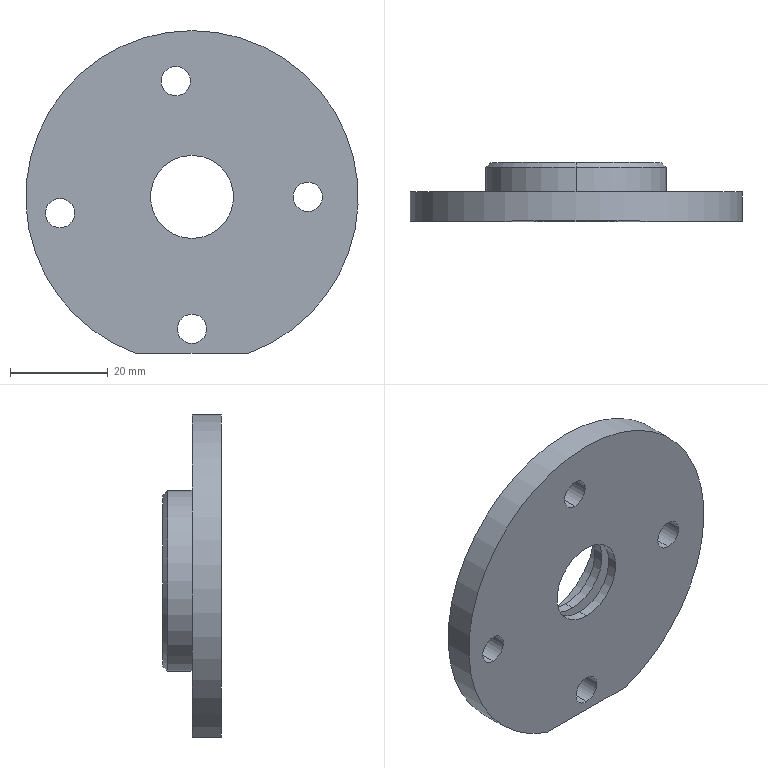Part | SolidWorks | features ICE 7, Chamfer 1, Extrusion 1, Fillet 1 | 1 solid | 30 faces | box 68 x 12 x 66 mm | volume 21544 mm3 | cylinder 19 | plane 7 | torus 2 | cone 2 | commonest cylinder face diameters 6 x8 17 x4 25 x2 29 x2 37 x2 68 x1
STEP:
#1=CARTESIAN_POINT('',(0.,0.,-30.));
#2=VERTEX_POINT('',#1);
#3=CARTESIAN_POINT('',(0.,0.,-24.));
#4=VERTEX_POINT('',#3);
#5=CARTESIAN_POINT('',(0.,0.,-27.));
#6=DIRECTION('',(0.,1.,0.));
#7=DIRECTION('',(0.,0.,1.));
#8=AXIS2_PLACEMENT_3D('',#5,#6,#7);
#9=CIRCLE('',#8,3.);
#10=EDGE_CURVE('',#2,#4,#9,.T.);
#11=ORIENTED_EDGE('',*,*,#10,.F.);
#12=CARTESIAN_POINT('',(0.,6.,-30.));
#13=VERTEX_POINT('',#12);
#14=CARTESIAN_POINT('',(0.,-74.,-30.));
#15=DIRECTION('',(0.,1.,0.));
#16=VECTOR('',#15,1000.);
#17=LINE('',#14,#16);
#18=EDGE_CURVE('',#2,#13,#17,.T.);
#19=ORIENTED_EDGE('',*,*,#18,.T.);
#20=CARTESIAN_POINT('',(0.,6.,-24.));
#21=VERTEX_POINT('',#20);
#22=CARTESIAN_POINT('',(0.,6.,-27.));
#23=DIRECTION('',(0.,1.,0.));
#24=DIRECTION('',(0.,0.,1.));
#25=AXIS2_PLACEMENT_3D('',#22,#23,#24);
#26=CIRCLE('',#25,3.);
#27=EDGE_CURVE('',#13,#21,#26,.T.);
#28=ORIENTED_EDGE('',*,*,#27,.T.);
#29=CARTESIAN_POINT('',(0.,-74.,-24.));
#30=DIRECTION('',(0.,1.,0.));
#31=VECTOR('',#30,1000.);
#32=LINE('',#29,#31);
#33=EDGE_CURVE('',#4,#21,#32,.T.);
#34=ORIENTED_EDGE('',*,*,#33,.F.);
#35=EDGE_LOOP('',(#11,#19,#28,#34));
#36=FACE_OUTER_BOUND('',#35,.T.);
#37=CARTESIAN_POINT('',(0.,-74.,-27.));
#38=DIRECTION('',(0.,1.,0.));
#39=DIRECTION('',(0.,0.,1.));
#40=AXIS2_PLACEMENT_3D('',#37,#38,#39);
#41=CYLINDRICAL_SURFACE('',#40,3.);
#42=ADVANCED_FACE('',(#36),#41,.F.);
#43=CARTESIAN_POINT('',(23.68,0.,-3.));
#44=VERTEX_POINT('',#43);
#45=CARTESIAN_POINT('',(23.68,0.,3.));
#46=VERTEX_POINT('',#45);
#47=CARTESIAN_POINT('',(23.68,0.,0.));
#48=DIRECTION('',(0.,1.,0.));
#49=DIRECTION('',(0.,0.,1.));
#50=AXIS2_PLACEMENT_3D('',#47,#48,#49);
#51=CIRCLE('',#50,3.);
#52=EDGE_CURVE('',#44,#46,#51,.T.);
#53=ORIENTED_EDGE('',*,*,#52,.F.);
#54=CARTESIAN_POINT('',(23.68,6.,-3.));
#55=VERTEX_POINT('',#54);
#56=CARTESIAN_POINT('',(23.68,-74.,-3.));
#57=DIRECTION('',(0.,1.,0.));
#58=VECTOR('',#57,1000.);
#59=LINE('',#56,#58);
#60=EDGE_CURVE('',#44,#55,#59,.T.);
#61=ORIENTED_EDGE('',*,*,#60,.T.);
#62=CARTESIAN_POINT('',(23.68,6.,3.));
#63=VERTEX_POINT('',#62);
#64=CARTESIAN_POINT('',(23.68,6.,0.));
#65=DIRECTION('',(0.,1.,0.));
#66=DIRECTION('',(0.,0.,1.));
#67=AXIS2_PLACEMENT_3D('',#64,#65,#66);
#68=CIRCLE('',#67,3.);
#69=EDGE_CURVE('',#55,#63,#68,.T.);
#70=ORIENTED_EDGE('',*,*,#69,.T.);
#71=CARTESIAN_POINT('',(23.68,-74.,3.));
#72=DIRECTION('',(0.,1.,0.));
#73=VECTOR('',#72,1000.);
#74=LINE('',#71,#73);
#75=EDGE_CURVE('',#46,#63,#74,.T.);
#76=ORIENTED_EDGE('',*,*,#75,.F.);
#77=EDGE_LOOP('',(#53,#61,#70,#76));
#78=FACE_OUTER_BOUND('',#77,.T.);
#79=CARTESIAN_POINT('',(23.68,-74.,0.));
#80=DIRECTION('',(0.,1.,0.));
#81=DIRECTION('',(0.,0.,1.));
#82=AXIS2_PLACEMENT_3D('',#79,#80,#81);
#83=CYLINDRICAL_SURFACE('',#82,3.);
#84=ADVANCED_FACE('',(#78),#83,.F.);
#85=CARTESIAN_POINT('',(-3.32,0.,20.68));
#86=VERTEX_POINT('',#85);
#87=CARTESIAN_POINT('',(-3.32,0.,26.68));
#88=VERTEX_POINT('',#87);
#89=CARTESIAN_POINT('',(-3.32,0.,23.68));
#90=DIRECTION('',(0.,1.,0.));
#91=DIRECTION('',(0.,0.,1.));
#92=AXIS2_PLACEMENT_3D('',#89,#90,#91);
#93=CIRCLE('',#92,3.);
#94=EDGE_CURVE('',#86,#88,#93,.T.);
#95=ORIENTED_EDGE('',*,*,#94,.F.);
#96=CARTESIAN_POINT('',(-3.32,6.,20.68));
#97=VERTEX_POINT('',#96);
#98=CARTESIAN_POINT('',(-3.32,-74.,20.68));
#99=DIRECTION('',(0.,1.,0.));
#100=VECTOR('',#99,1000.);
#101=LINE('',#98,#100);
#102=EDGE_CURVE('',#86,#97,#101,.T.);
#103=ORIENTED_EDGE('',*,*,#102,.T.);
#104=CARTESIAN_POINT('',(-3.32,6.,26.68));
#105=VERTEX_POINT('',#104);
#106=CARTESIAN_POINT('',(-3.32,6.,23.68));
#107=DIRECTION('',(0.,1.,0.));
#108=DIRECTION('',(0.,0.,1.));
#109=AXIS2_PLACEMENT_3D('',#106,#107,#108);
#110=CIRCLE('',#109,3.);
#111=EDGE_CURVE('',#97,#105,#110,.T.);
#112=ORIENTED_EDGE('',*,*,#111,.T.);
#113=CARTESIAN_POINT('',(-3.32,-74.,26.68));
#114=DIRECTION('',(0.,1.,0.));
#115=VECTOR('',#114,1000.);
#116=LINE('',#113,#115);
#117=EDGE_CURVE('',#88,#105,#116,.T.);
#118=ORIENTED_EDGE('',*,*,#117,.F.);
#119=EDGE_LOOP('',(#95,#103,#112,#118));
#120=FACE_OUTER_BOUND('',#119,.T.);
#121=CARTESIAN_POINT('',(-3.32,-74.,23.68));
#122=DIRECTION('',(0.,1.,0.));
#123=DIRECTION('',(0.,0.,1.));
#124=AXIS2_PLACEMENT_3D('',#121,#122,#123);
#125=CYLINDRICAL_SURFACE('',#124,3.);
#126=ADVANCED_FACE('',(#120),#125,.F.);
#127=CARTESIAN_POINT('',(-27.,0.,-6.32));
#128=VERTEX_POINT('',#127);
#129=CARTESIAN_POINT('',(-27.,0.,-0.32));
#130=VERTEX_POINT('',#129);
#131=CARTESIAN_POINT('',(-27.,0.,-3.32));
#132=DIRECTION('',(0.,1.,0.));
#133=DIRECTION('',(0.,0.,1.));
#134=AXIS2_PLACEMENT_3D('',#131,#132,#133);
#135=CIRCLE('',#134,3.);
#136=EDGE_CURVE('',#128,#130,#135,.T.);
#137=ORIENTED_EDGE('',*,*,#136,.F.);
#138=CARTESIAN_POINT('',(-27.,6.,-6.32));
#139=VERTEX_POINT('',#138);
#140=CARTESIAN_POINT('',(-27.,-74.,-6.32));
#141=DIRECTION('',(0.,1.,0.));
#142=VECTOR('',#141,1000.);
#143=LINE('',#140,#142);
#144=EDGE_CURVE('',#128,#139,#143,.T.);
#145=ORIENTED_EDGE('',*,*,#144,.T.);
#146=CARTESIAN_POINT('',(-27.,6.,-0.32));
#147=VERTEX_POINT('',#146);
#148=CARTESIAN_POINT('',(-27.,6.,-3.32));
#149=DIRECTION('',(0.,1.,0.));
#150=DIRECTION('',(0.,0.,1.));
#151=AXIS2_PLACEMENT_3D('',#148,#149,#150);
#152=CIRCLE('',#151,3.);
#153=EDGE_CURVE('',#139,#147,#152,.T.);
#154=ORIENTED_EDGE('',*,*,#153,.T.);
#155=CARTESIAN_POINT('',(-27.,-74.,-0.32));
#156=DIRECTION('',(0.,1.,0.));
#157=VECTOR('',#156,1000.);
#158=LINE('',#155,#157);
#159=EDGE_CURVE('',#130,#147,#158,.T.);
#160=ORIENTED_EDGE('',*,*,#159,.F.);
#161=EDGE_LOOP('',(#137,#145,#154,#160));
#162=FACE_OUTER_BOUND('',#161,.T.);
#163=CARTESIAN_POINT('',(-27.,-74.,-3.32));
#164=DIRECTION('',(0.,1.,0.));
#165=DIRECTION('',(0.,0.,1.));
#166=AXIS2_PLACEMENT_3D('',#163,#164,#165);
#167=CYLINDRICAL_SURFACE('',#166,3.);
#168=ADVANCED_FACE('',(#162),#167,.F.);
#169=CARTESIAN_POINT('',(0.,6.,-12.5));
#170=VERTEX_POINT('',#169);
#171=CARTESIAN_POINT('',(0.,6.,12.5));
#172=VERTEX_POINT('',#171);
#173=CARTESIAN_POINT('',(0.,6.,0.));
#174=DIRECTION('',(0.,1.,0.));
#175=DIRECTION('',(0.,0.,1.));
#176=AXIS2_PLACEMENT_3D('',#173,#174,#175);
#177=CIRCLE('',#176,12.5);
#178=EDGE_CURVE('',#170,#172,#177,.T.);
#179=ORIENTED_EDGE('',*,*,#178,.F.);
#180=CARTESIAN_POINT('',(0.,8.,-14.5));
#181=VERTEX_POINT('',#180);
#182=CARTESIAN_POINT('',(0.,8.,-12.5));
#183=DIRECTION('',(1.,0.,0.));
#184=DIRECTION('',(0.,0.,-1.));
#185=AXIS2_PLACEMENT_3D('',#182,#183,#184);
#186=CIRCLE('',#185,2.);
#187=EDGE_CURVE('',#170,#181,#186,.T.);
#188=ORIENTED_EDGE('',*,*,#187,.T.);
#189=CARTESIAN_POINT('',(0.,8.,14.5));
#190=VERTEX_POINT('',#189);
#191=CARTESIAN_POINT('',(0.,8.,0.));
#192=DIRECTION('',(0.,-1.,0.));
#193=DIRECTION('',(0.,0.,1.));
#194=AXIS2_PLACEMENT_3D('',#191,#192,#193);
#195=CIRCLE('',#194,14.5);
#196=EDGE_CURVE('',#190,#181,#195,.T.);
#197=ORIENTED_EDGE('',*,*,#196,.F.);
#198=CARTESIAN_POINT('',(0.,8.,12.5));
#199=DIRECTION('',(-1.,0.,0.));
#200=DIRECTION('',(0.,0.,1.));
#201=AXIS2_PLACEMENT_3D('',#198,#199,#200);
#202=CIRCLE('',#201,2.);
#203=EDGE_CURVE('',#172,#190,#202,.T.);
#204=ORIENTED_EDGE('',*,*,#203,.F.);
#205=EDGE_LOOP('',(#179,#188,#197,#204));
#206=FACE_OUTER_BOUND('',#205,.T.);
#207=CARTESIAN_POINT('',(0.,8.,0.));
#208=DIRECTION('',(0.,1.,0.));
#209=DIRECTION('',(0.,0.,1.));
#210=AXIS2_PLACEMENT_3D('',#207,#208,#209);
#211=TOROIDAL_SURFACE('',#210,12.5,2.);
#212=ADVANCED_FACE('',(#206),#211,.F.);
#213=CARTESIAN_POINT('',(0.,12.,17.5));
#214=VERTEX_POINT('',#213);
#215=CARTESIAN_POINT('',(0.,12.,-17.5));
#216=VERTEX_POINT('',#215);
#217=CARTESIAN_POINT('',(0.,12.,0.));
#218=DIRECTION('',(0.,1.,0.));
#219=DIRECTION('',(0.,0.,1.));
#220=AXIS2_PLACEMENT_3D('',#217,#218,#219);
#221=CIRCLE('',#220,17.5);
#222=EDGE_CURVE('',#214,#216,#221,.T.);
#223=ORIENTED_EDGE('',*,*,#222,.F.);
#224=CARTESIAN_POINT('',(0.,11.,18.5));
#225=VERTEX_POINT('',#224);
#226=CARTESIAN_POINT('',(0.,12.,17.5));
#227=DIRECTION('',(0.,-0.7071,0.7071));
#228=VECTOR('',#227,1000.);
#229=LINE('',#226,#228);
#230=EDGE_CURVE('',#214,#225,#229,.T.);
#231=ORIENTED_EDGE('',*,*,#230,.T.);
#232=CARTESIAN_POINT('',(0.,11.,-18.5));
#233=VERTEX_POINT('',#232);
#234=CARTESIAN_POINT('',(0.,11.,0.));
#235=DIRECTION('',(0.,-1.,0.));
#236=DIRECTION('',(0.,0.,1.));
#237=AXIS2_PLACEMENT_3D('',#234,#235,#236);
#238=CIRCLE('',#237,18.5);
#239=EDGE_CURVE('',#233,#225,#238,.T.);
#240=ORIENTED_EDGE('',*,*,#239,.F.);
#241=CARTESIAN_POINT('',(0.,12.,-17.5));
#242=DIRECTION('',(0.,-0.7071,-0.7071));
#243=VECTOR('',#242,1000.);
#244=LINE('',#241,#243);
#245=EDGE_CURVE('',#216,#233,#244,.T.);
#246=ORIENTED_EDGE('',*,*,#245,.F.);
#247=EDGE_LOOP('',(#223,#231,#240,#246));
#248=FACE_OUTER_BOUND('',#247,.T.);
#249=CARTESIAN_POINT('',(0.,12.,0.));
#250=DIRECTION('',(0.,-1.,0.));
#251=DIRECTION('',(0.,0.,-1.));
#252=AXIS2_PLACEMENT_3D('',#249,#250,#251);
#253=CONICAL_SURFACE('',#252,17.5,0.7854);
#254=ADVANCED_FACE('',(#248),#253,.T.);
#255=CARTESIAN_POINT('',(0.,0.,-8.5));
#256=VERTEX_POINT('',#255);
#257=CARTESIAN_POINT('',(0.,0.,8.5));
#258=VERTEX_POINT('',#257);
#259=CARTESIAN_POINT('',(0.,0.,0.));
#260=DIRECTION('',(0.,1.,0.));
#261=DIRECTION('',(0.,0.,1.));
#262=AXIS2_PLACEMENT_3D('',#259,#260,#261);
#263=CIRCLE('',#262,8.5);
#264=EDGE_CURVE('',#256,#258,#263,.T.);
#265=ORIENTED_EDGE('',*,*,#264,.F.);
#266=CARTESIAN_POINT('',(0.,2.,-8.5));
#267=VERTEX_POINT('',#266);
#268=CARTESIAN_POINT('',(0.,0.,-8.5));
#269=DIRECTION('',(0.,1.,0.));
#270=VECTOR('',#269,1000.);
#271=LINE('',#268,#270);
#272=EDGE_CURVE('',#256,#267,#271,.T.);
#273=ORIENTED_EDGE('',*,*,#272,.T.);
#274=CARTESIAN_POINT('',(0.,2.,8.5));
#275=VERTEX_POINT('',#274);
#276=CARTESIAN_POINT('',(0.,2.,0.));
#277=DIRECTION('',(0.,1.,0.));
#278=DIRECTION('',(0.,0.,1.));
#279=AXIS2_PLACEMENT_3D('',#276,#277,#278);
#280=CIRCLE('',#279,8.5);
#281=EDGE_CURVE('',#267,#275,#280,.T.);
#282=ORIENTED_EDGE('',*,*,#281,.T.);
#283=CARTESIAN_POINT('',(0.,0.,8.5));
#284=DIRECTION('',(0.,1.,0.));
#285=VECTOR('',#284,1000.);
#286=LINE('',#283,#285);
#287=EDGE_CURVE('',#258,#275,#286,.T.);
#288=ORIENTED_EDGE('',*,*,#287,.F.);
#289=EDGE_LOOP('',(#265,#273,#282,#288));
#290=FACE_OUTER_BOUND('',#289,.T.);
#291=CARTESIAN_POINT('',(0.,0.,0.));
#292=DIRECTION('',(0.,1.,0.));
#293=DIRECTION('',(0.,0.,1.));
#294=AXIS2_PLACEMENT_3D('',#291,#292,#293);
#295=CYLINDRICAL_SURFACE('',#294,8.5);
#296=ADVANCED_FACE('',(#290),#295,.F.);
#297=CARTESIAN_POINT('',(0.,2.,-12.5));
#298=VERTEX_POINT('',#297);
#299=CARTESIAN_POINT('',(0.,2.,12.5));
#300=VERTEX_POINT('',#299);
#301=CARTESIAN_POINT('',(0.,2.,0.));
#302=DIRECTION('',(0.,1.,0.));
#303=DIRECTION('',(0.,0.,1.));
#304=AXIS2_PLACEMENT_3D('',#301,#302,#303);
#305=CIRCLE('',#304,12.5);
#306=EDGE_CURVE('',#298,#300,#305,.T.);
#307=ORIENTED_EDGE('',*,*,#306,.F.);
#308=CARTESIAN_POINT('',(0.,4.,-12.5));
#309=VERTEX_POINT('',#308);
#310=CARTESIAN_POINT('',(0.,2.,-12.5));
#311=DIRECTION('',(0.,1.,0.));
#312=VECTOR('',#311,1000.);
#313=LINE('',#310,#312);
#314=EDGE_CURVE('',#298,#309,#313,.T.);
#315=ORIENTED_EDGE('',*,*,#314,.T.);
#316=CARTESIAN_POINT('',(0.,4.,12.5));
#317=VERTEX_POINT('',#316);
#318=CARTESIAN_POINT('',(0.,4.,0.));
#319=DIRECTION('',(0.,1.,0.));
#320=DIRECTION('',(0.,0.,1.));
#321=AXIS2_PLACEMENT_3D('',#318,#319,#320);
#322=CIRCLE('',#321,12.5);
#323=EDGE_CURVE('',#309,#317,#322,.T.);
#324=ORIENTED_EDGE('',*,*,#323,.T.);
#325=CARTESIAN_POINT('',(0.,2.,12.5));
#326=DIRECTION('',(0.,1.,0.));
#327=VECTOR('',#326,1000.);
#328=LINE('',#325,#327);
#329=EDGE_CURVE('',#300,#317,#328,.T.);
#330=ORIENTED_EDGE('',*,*,#329,.F.);
#331=EDGE_LOOP('',(#307,#315,#324,#330));
#332=FACE_OUTER_BOUND('',#331,.T.);
#333=CARTESIAN_POINT('',(0.,2.,0.));
#334=DIRECTION('',(0.,1.,0.));
#335=DIRECTION('',(0.,0.,1.));
#336=AXIS2_PLACEMENT_3D('',#333,#334,#335);
#337=CYLINDRICAL_SURFACE('',#336,12.5);
#338=ADVANCED_FACE('',(#332),#337,.F.);
#339=CARTESIAN_POINT('',(0.,4.,-8.5));
#340=VERTEX_POINT('',#339);
#341=CARTESIAN_POINT('',(0.,4.,8.5));
#342=VERTEX_POINT('',#341);
#343=CARTESIAN_POINT('',(0.,4.,0.));
#344=DIRECTION('',(0.,1.,0.));
#345=DIRECTION('',(0.,0.,1.));
#346=AXIS2_PLACEMENT_3D('',#343,#344,#345);
#347=CIRCLE('',#346,8.5);
#348=EDGE_CURVE('',#340,#342,#347,.T.);
#349=ORIENTED_EDGE('',*,*,#348,.F.);
#350=CARTESIAN_POINT('',(0.,6.,-8.5));
#351=VERTEX_POINT('',#350);
#352=CARTESIAN_POINT('',(0.,4.,-8.5));
#353=DIRECTION('',(0.,1.,0.));
#354=VECTOR('',#353,1000.);
#355=LINE('',#352,#354);
#356=EDGE_CURVE('',#340,#351,#355,.T.);
#357=ORIENTED_EDGE('',*,*,#356,.T.);
#358=CARTESIAN_POINT('',(0.,6.,8.5));
#359=VERTEX_POINT('',#358);
#360=CARTESIAN_POINT('',(0.,6.,0.));
#361=DIRECTION('',(0.,1.,0.));
#362=DIRECTION('',(0.,0.,1.));
#363=AXIS2_PLACEMENT_3D('',#360,#361,#362);
#364=CIRCLE('',#363,8.5);
#365=EDGE_CURVE('',#351,#359,#364,.T.);
#366=ORIENTED_EDGE('',*,*,#365,.T.);
#367=CARTESIAN_POINT('',(0.,4.,8.5));
#368=DIRECTION('',(0.,1.,0.));
#369=VECTOR('',#368,1000.);
#370=LINE('',#367,#369);
#371=EDGE_CURVE('',#342,#359,#370,.T.);
#372=ORIENTED_EDGE('',*,*,#371,.F.);
#373=EDGE_LOOP('',(#349,#357,#366,#372));
#374=FACE_OUTER_BOUND('',#373,.T.);
#375=CARTESIAN_POINT('',(0.,4.,0.));
#376=DIRECTION('',(0.,1.,0.));
#377=DIRECTION('',(0.,0.,1.));
#378=AXIS2_PLACEMENT_3D('',#375,#376,#377);
#379=CYLINDRICAL_SURFACE('',#378,8.5);
#380=ADVANCED_FACE('',(#374),#379,.F.);
#381=ORIENTED_EDGE('',*,*,#196,.T.);
#382=CARTESIAN_POINT('',(0.,12.,-14.5));
#383=VERTEX_POINT('',#382);
#384=CARTESIAN_POINT('',(0.,6.,-14.5));
#385=DIRECTION('',(0.,1.,0.));
#386=VECTOR('',#385,1000.);
#387=LINE('',#384,#386);
#388=EDGE_CURVE('',#181,#383,#387,.T.);
#389=ORIENTED_EDGE('',*,*,#388,.T.);
#390=CARTESIAN_POINT('',(0.,12.,14.5));
#391=VERTEX_POINT('',#390);
#392=CARTESIAN_POINT('',(0.,12.,0.));
#393=DIRECTION('',(0.,1.,0.));
#394=DIRECTION('',(0.,0.,1.));
#395=AXIS2_PLACEMENT_3D('',#392,#393,#394);
#396=CIRCLE('',#395,14.5);
#397=EDGE_CURVE('',#383,#391,#396,.T.);
#398=ORIENTED_EDGE('',*,*,#397,.T.);
#399=CARTESIAN_POINT('',(0.,6.,14.5));
#400=DIRECTION('',(0.,1.,0.));
#401=VECTOR('',#400,1000.);
#402=LINE('',#399,#401);
#403=EDGE_CURVE('',#190,#391,#402,.T.);
#404=ORIENTED_EDGE('',*,*,#403,.F.);
#405=EDGE_LOOP('',(#381,#389,#398,#404));
#406=FACE_OUTER_BOUND('',#405,.T.);
#407=CARTESIAN_POINT('',(0.,6.,0.));
#408=DIRECTION('',(0.,1.,0.));
#409=DIRECTION('',(0.,0.,1.));
#410=AXIS2_PLACEMENT_3D('',#407,#408,#409);
#411=CYLINDRICAL_SURFACE('',#410,14.5);
#412=ADVANCED_FACE('',(#406),#411,.F.);
#413=ORIENTED_EDGE('',*,*,#239,.T.);
#414=CARTESIAN_POINT('',(0.,6.,18.5));
#415=VERTEX_POINT('',#414);
#416=CARTESIAN_POINT('',(0.,12.,18.5));
#417=DIRECTION('',(0.,-1.,0.));
#418=VECTOR('',#417,1000.);
#419=LINE('',#416,#418);
#420=EDGE_CURVE('',#225,#415,#419,.T.);
#421=ORIENTED_EDGE('',*,*,#420,.T.);
#422=CARTESIAN_POINT('',(0.,6.,-18.5));
#423=VERTEX_POINT('',#422);
#424=CARTESIAN_POINT('',(0.,6.,0.));
#425=DIRECTION('',(0.,1.,0.));
#426=DIRECTION('',(0.,0.,1.));
#427=AXIS2_PLACEMENT_3D('',#424,#425,#426);
#428=CIRCLE('',#427,18.5);
#429=EDGE_CURVE('',#415,#423,#428,.T.);
#430=ORIENTED_EDGE('',*,*,#429,.T.);
#431=CARTESIAN_POINT('',(0.,12.,-18.5));
#432=DIRECTION('',(0.,-1.,0.));
#433=VECTOR('',#432,1000.);
#434=LINE('',#431,#433);
#435=EDGE_CURVE('',#233,#423,#434,.T.);
#436=ORIENTED_EDGE('',*,*,#435,.F.);
#437=EDGE_LOOP('',(#413,#421,#430,#436));
#438=FACE_OUTER_BOUND('',#437,.T.);
#439=CARTESIAN_POINT('',(0.,12.,0.));
#440=DIRECTION('',(0.,-1.,0.));
#441=DIRECTION('',(0.,0.,-1.));
#442=AXIS2_PLACEMENT_3D('',#439,#440,#441);
#443=CYLINDRICAL_SURFACE('',#442,18.5);
#444=ADVANCED_FACE('',(#438),#443,.T.);
#445=CARTESIAN_POINT('',(-11.489,6.,-32.));
#446=VERTEX_POINT('',#445);
#447=CARTESIAN_POINT('',(11.489,6.,-32.));
#448=VERTEX_POINT('',#447);
#449=CARTESIAN_POINT('',(0.,6.,0.));
#450=DIRECTION('',(0.,1.,0.));
#451=DIRECTION('',(0.,0.,1.));
#452=AXIS2_PLACEMENT_3D('',#449,#450,#451);
#453=CIRCLE('',#452,34.);
#454=EDGE_CURVE('',#446,#448,#453,.T.);
#455=ORIENTED_EDGE('',*,*,#454,.F.);
#456=CARTESIAN_POINT('',(-11.489,0.,-32.));
#457=VERTEX_POINT('',#456);
#458=CARTESIAN_POINT('',(-11.489,6.,-32.));
#459=DIRECTION('',(0.,-1.,0.));
#460=VECTOR('',#459,1000.);
#461=LINE('',#458,#460);
#462=EDGE_CURVE('',#446,#457,#461,.T.);
#463=ORIENTED_EDGE('',*,*,#462,.T.);
#464=CARTESIAN_POINT('',(11.489,0.,-32.));
#465=VERTEX_POINT('',#464);
#466=CARTESIAN_POINT('',(0.,0.,0.));
#467=DIRECTION('',(0.,1.,0.));
#468=DIRECTION('',(0.,0.,1.));
#469=AXIS2_PLACEMENT_3D('',#466,#467,#468);
#470=CIRCLE('',#469,34.);
#471=EDGE_CURVE('',#457,#465,#470,.T.);
#472=ORIENTED_EDGE('',*,*,#471,.T.);
#473=CARTESIAN_POINT('',(11.489,6.,-32.));
#474=DIRECTION('',(0.,1.,0.));
#475=VECTOR('',#474,1000.);
#476=LINE('',#473,#475);
#477=EDGE_CURVE('',#465,#448,#476,.T.);
#478=ORIENTED_EDGE('',*,*,#477,.T.);
#479=EDGE_LOOP('',(#455,#463,#472,#478));
#480=FACE_OUTER_BOUND('',#479,.T.);
#481=CARTESIAN_POINT('',(0.,6.,0.));
#482=DIRECTION('',(0.,-1.,0.));
#483=DIRECTION('',(0.,0.,-1.));
#484=AXIS2_PLACEMENT_3D('',#481,#482,#483);
#485=CYLINDRICAL_SURFACE('',#484,34.);
#486=ADVANCED_FACE('',(#480),#485,.T.);
#487=CARTESIAN_POINT('',(0.,6.,-27.));
#488=DIRECTION('',(0.,1.,0.));
#489=DIRECTION('',(0.,0.,1.));
#490=AXIS2_PLACEMENT_3D('',#487,#488,#489);
#491=CIRCLE('',#490,3.);
#492=EDGE_CURVE('',#21,#13,#491,.T.);
#493=ORIENTED_EDGE('',*,*,#492,.F.);
#494=ORIENTED_EDGE('',*,*,#27,.F.);
#495=EDGE_LOOP('',(#493,#494));
#496=FACE_BOUND('',#495,.T.);
#497=CARTESIAN_POINT('',(23.68,6.,0.));
#498=DIRECTION('',(0.,1.,0.));
#499=DIRECTION('',(0.,0.,1.));
#500=AXIS2_PLACEMENT_3D('',#497,#498,#499);
#501=CIRCLE('',#500,3.);
#502=EDGE_CURVE('',#63,#55,#501,.T.);
#503=ORIENTED_EDGE('',*,*,#502,.F.);
#504=ORIENTED_EDGE('',*,*,#69,.F.);
#505=EDGE_LOOP('',(#503,#504));
#506=FACE_BOUND('',#505,.T.);
#507=CARTESIAN_POINT('',(-3.32,6.,23.68));
#508=DIRECTION('',(0.,1.,0.));
#509=DIRECTION('',(0.,0.,1.));
#510=AXIS2_PLACEMENT_3D('',#507,#508,#509);
#511=CIRCLE('',#510,3.);
#512=EDGE_CURVE('',#105,#97,#511,.T.);
#513=ORIENTED_EDGE('',*,*,#512,.F.);
#514=ORIENTED_EDGE('',*,*,#111,.F.);
#515=EDGE_LOOP('',(#513,#514));
#516=FACE_BOUND('',#515,.T.);
#517=CARTESIAN_POINT('',(-27.,6.,-3.32));
#518=DIRECTION('',(0.,1.,0.));
#519=DIRECTION('',(0.,0.,1.));
#520=AXIS2_PLACEMENT_3D('',#517,#518,#519);
#521=CIRCLE('',#520,3.);
#522=EDGE_CURVE('',#147,#139,#521,.T.);
#523=ORIENTED_EDGE('',*,*,#522,.F.);
#524=ORIENTED_EDGE('',*,*,#153,.F.);
#525=EDGE_LOOP('',(#523,#524));
#526=FACE_BOUND('',#525,.T.);
#527=CARTESIAN_POINT('',(-19.623,6.,-32.));
#528=DIRECTION('',(1.,0.,0.));
#529=VECTOR('',#528,1000.);
#530=LINE('',#527,#529);
#531=EDGE_CURVE('',#446,#448,#530,.T.);
#532=ORIENTED_EDGE('',*,*,#531,.F.);
#533=ORIENTED_EDGE('',*,*,#454,.T.);
#534=EDGE_LOOP('',(#532,#533));
#535=FACE_OUTER_BOUND('',#534,.T.);
#536=CARTESIAN_POINT('',(0.,6.,0.));
#537=DIRECTION('',(0.,1.,0.));
#538=DIRECTION('',(0.,0.,1.));
#539=AXIS2_PLACEMENT_3D('',#536,#537,#538);
#540=CIRCLE('',#539,18.5);
#541=EDGE_CURVE('',#423,#415,#540,.T.);
#542=ORIENTED_EDGE('',*,*,#541,.F.);
#543=ORIENTED_EDGE('',*,*,#429,.F.);
#544=EDGE_LOOP('',(#542,#543));
#545=FACE_BOUND('',#544,.T.);
#546=CARTESIAN_POINT('',(0.,6.,0.));
#547=DIRECTION('',(0.,1.,0.));
#548=DIRECTION('',(0.,0.,1.));
#549=AXIS2_PLACEMENT_3D('',#546,#547,#548);
#550=PLANE('',#549);
#551=ADVANCED_FACE('',(#496,#506,#516,#526,#535,#545),#550,.T.);
#552=CARTESIAN_POINT('',(0.,0.,-27.));
#553=DIRECTION('',(0.,1.,0.));
#554=DIRECTION('',(0.,0.,1.));
#555=AXIS2_PLACEMENT_3D('',#552,#553,#554);
#556=CIRCLE('',#555,3.);
#557=EDGE_CURVE('',#4,#2,#556,.T.);
#558=ORIENTED_EDGE('',*,*,#557,.T.);
#559=ORIENTED_EDGE('',*,*,#10,.T.);
#560=EDGE_LOOP('',(#558,#559));
#561=FACE_BOUND('',#560,.T.);
#562=CARTESIAN_POINT('',(23.68,0.,0.));
#563=DIRECTION('',(0.,1.,0.));
#564=DIRECTION('',(0.,0.,1.));
#565=AXIS2_PLACEMENT_3D('',#562,#563,#564);
#566=CIRCLE('',#565,3.);
#567=EDGE_CURVE('',#46,#44,#566,.T.);
#568=ORIENTED_EDGE('',*,*,#567,.T.);
#569=ORIENTED_EDGE('',*,*,#52,.T.);
#570=EDGE_LOOP('',(#568,#569));
#571=FACE_BOUND('',#570,.T.);
#572=CARTESIAN_POINT('',(-3.32,0.,23.68));
#573=DIRECTION('',(0.,1.,0.));
#574=DIRECTION('',(0.,0.,1.));
#575=AXIS2_PLACEMENT_3D('',#572,#573,#574);
#576=CIRCLE('',#575,3.);
#577=EDGE_CURVE('',#88,#86,#576,.T.);
#578=ORIENTED_EDGE('',*,*,#577,.T.);
#579=ORIENTED_EDGE('',*,*,#94,.T.);
#580=EDGE_LOOP('',(#578,#579));
#581=FACE_BOUND('',#580,.T.);
#582=CARTESIAN_POINT('',(-27.,0.,-3.32));
#583=DIRECTION('',(0.,1.,0.));
#584=DIRECTION('',(0.,0.,1.));
#585=AXIS2_PLACEMENT_3D('',#582,#583,#584);
#586=CIRCLE('',#585,3.);
#587=EDGE_CURVE('',#130,#128,#586,.T.);
#588=ORIENTED_EDGE('',*,*,#587,.T.);
#589=ORIENTED_EDGE('',*,*,#136,.T.);
#590=EDGE_LOOP('',(#588,#589));
#591=FACE_BOUND('',#590,.T.);
#592=CARTESIAN_POINT('',(0.,0.,0.));
#593=DIRECTION('',(0.,1.,0.));
#594=DIRECTION('',(0.,0.,1.));
#595=AXIS2_PLACEMENT_3D('',#592,#593,#594);
#596=CIRCLE('',#595,8.5);
#597=EDGE_CURVE('',#258,#256,#596,.T.);
#598=ORIENTED_EDGE('',*,*,#597,.T.);
#599=ORIENTED_EDGE('',*,*,#264,.T.);
#600=EDGE_LOOP('',(#598,#599));
#601=FACE_BOUND('',#600,.T.);
#602=ORIENTED_EDGE('',*,*,#471,.F.);
#603=CARTESIAN_POINT('',(0.,0.,-32.));
#604=DIRECTION('',(1.,0.,0.));
#605=VECTOR('',#604,1000.);
#606=LINE('',#603,#605);
#607=EDGE_CURVE('',#457,#465,#606,.T.);
#608=ORIENTED_EDGE('',*,*,#607,.T.);
#609=EDGE_LOOP('',(#602,#608));
#610=FACE_OUTER_BOUND('',#609,.T.);
#611=CARTESIAN_POINT('',(0.,0.,0.));
#612=DIRECTION('',(0.,1.,0.));
#613=DIRECTION('',(0.,0.,1.));
#614=AXIS2_PLACEMENT_3D('',#611,#612,#613);
#615=PLANE('',#614);
#616=ADVANCED_FACE('',(#561,#571,#581,#591,#601,#610),#615,.F.);
#617=ORIENTED_EDGE('',*,*,#420,.F.);
#618=CARTESIAN_POINT('',(0.,11.,0.));
#619=DIRECTION('',(0.,-1.,0.));
#620=DIRECTION('',(0.,0.,1.));
#621=AXIS2_PLACEMENT_3D('',#618,#619,#620);
#622=CIRCLE('',#621,18.5);
#623=EDGE_CURVE('',#225,#233,#622,.T.);
#624=ORIENTED_EDGE('',*,*,#623,.T.);
#625=ORIENTED_EDGE('',*,*,#435,.T.);
#626=ORIENTED_EDGE('',*,*,#541,.T.);
#627=EDGE_LOOP('',(#617,#624,#625,#626));
#628=FACE_OUTER_BOUND('',#627,.T.);
#629=CARTESIAN_POINT('',(0.,12.,0.));
#630=DIRECTION('',(0.,-1.,0.));
#631=DIRECTION('',(0.,0.,-1.));
#632=AXIS2_PLACEMENT_3D('',#629,#630,#631);
#633=CYLINDRICAL_SURFACE('',#632,18.5);
#634=ADVANCED_FACE('',(#628),#633,.T.);
#635=CARTESIAN_POINT('',(0.,12.,0.));
#636=DIRECTION('',(0.,1.,0.));
#637=DIRECTION('',(0.,0.,1.));
#638=AXIS2_PLACEMENT_3D('',#635,#636,#637);
#639=CIRCLE('',#638,17.5);
#640=EDGE_CURVE('',#216,#214,#639,.T.);
#641=ORIENTED_EDGE('',*,*,#640,.T.);
#642=ORIENTED_EDGE('',*,*,#222,.T.);
#643=EDGE_LOOP('',(#641,#642));
#644=FACE_OUTER_BOUND('',#643,.T.);
#645=CARTESIAN_POINT('',(0.,12.,0.));
#646=DIRECTION('',(0.,1.,0.));
#647=DIRECTION('',(0.,0.,1.));
#648=AXIS2_PLACEMENT_3D('',#645,#646,#647);
#649=CIRCLE('',#648,14.5);
#650=EDGE_CURVE('',#391,#383,#649,.T.);
#651=ORIENTED_EDGE('',*,*,#650,.F.);
#652=ORIENTED_EDGE('',*,*,#397,.F.);
#653=EDGE_LOOP('',(#651,#652));
#654=FACE_BOUND('',#653,.T.);
#655=CARTESIAN_POINT('',(0.,12.,0.));
#656=DIRECTION('',(0.,1.,0.));
#657=DIRECTION('',(0.,0.,1.));
#658=AXIS2_PLACEMENT_3D('',#655,#656,#657);
#659=PLANE('',#658);
#660=ADVANCED_FACE('',(#644,#654),#659,.T.);
#661=ORIENTED_EDGE('',*,*,#388,.F.);
#662=CARTESIAN_POINT('',(0.,8.,0.));
#663=DIRECTION('',(0.,-1.,0.));
#664=DIRECTION('',(0.,0.,1.));
#665=AXIS2_PLACEMENT_3D('',#662,#663,#664);
#666=CIRCLE('',#665,14.5);
#667=EDGE_CURVE('',#181,#190,#666,.T.);
#668=ORIENTED_EDGE('',*,*,#667,.T.);
#669=ORIENTED_EDGE('',*,*,#403,.T.);
#670=ORIENTED_EDGE('',*,*,#650,.T.);
#671=EDGE_LOOP('',(#661,#668,#669,#670));
#672=FACE_OUTER_BOUND('',#671,.T.);
#673=CARTESIAN_POINT('',(0.,6.,0.));
#674=DIRECTION('',(0.,1.,0.));
#675=DIRECTION('',(0.,0.,1.));
#676=AXIS2_PLACEMENT_3D('',#673,#674,#675);
#677=CYLINDRICAL_SURFACE('',#676,14.5);
#678=ADVANCED_FACE('',(#672),#677,.F.);
#679=CARTESIAN_POINT('',(0.,6.,0.));
#680=DIRECTION('',(0.,1.,0.));
#681=DIRECTION('',(0.,0.,1.));
#682=AXIS2_PLACEMENT_3D('',#679,#680,#681);
#683=CIRCLE('',#682,12.5);
#684=EDGE_CURVE('',#172,#170,#683,.T.);
#685=ORIENTED_EDGE('',*,*,#684,.T.);
#686=ORIENTED_EDGE('',*,*,#178,.T.);
#687=EDGE_LOOP('',(#685,#686));
#688=FACE_OUTER_BOUND('',#687,.T.);
#689=CARTESIAN_POINT('',(0.,6.,0.));
#690=DIRECTION('',(0.,1.,0.));
#691=DIRECTION('',(0.,0.,1.));
#692=AXIS2_PLACEMENT_3D('',#689,#690,#691);
#693=CIRCLE('',#692,8.5);
#694=EDGE_CURVE('',#359,#351,#693,.T.);
#695=ORIENTED_EDGE('',*,*,#694,.F.);
#696=ORIENTED_EDGE('',*,*,#365,.F.);
#697=EDGE_LOOP('',(#695,#696));
#698=FACE_BOUND('',#697,.T.);
#699=CARTESIAN_POINT('',(0.,6.,0.));
#700=DIRECTION('',(0.,1.,0.));
#701=DIRECTION('',(0.,0.,1.));
#702=AXIS2_PLACEMENT_3D('',#699,#700,#701);
#703=PLANE('',#702);
#704=ADVANCED_FACE('',(#688,#698),#703,.T.);
#705=ORIENTED_EDGE('',*,*,#356,.F.);
#706=CARTESIAN_POINT('',(0.,4.,0.));
#707=DIRECTION('',(0.,1.,0.));
#708=DIRECTION('',(0.,0.,1.));
#709=AXIS2_PLACEMENT_3D('',#706,#707,#708);
#710=CIRCLE('',#709,8.5);
#711=EDGE_CURVE('',#342,#340,#710,.T.);
#712=ORIENTED_EDGE('',*,*,#711,.F.);
#713=ORIENTED_EDGE('',*,*,#371,.T.);
#714=ORIENTED_EDGE('',*,*,#694,.T.);
#715=EDGE_LOOP('',(#705,#712,#713,#714));
#716=FACE_OUTER_BOUND('',#715,.T.);
#717=CARTESIAN_POINT('',(0.,4.,0.));
#718=DIRECTION('',(0.,1.,0.));
#719=DIRECTION('',(0.,0.,1.));
#720=AXIS2_PLACEMENT_3D('',#717,#718,#719);
#721=CYLINDRICAL_SURFACE('',#720,8.5);
#722=ADVANCED_FACE('',(#716),#721,.F.);
#723=ORIENTED_EDGE('',*,*,#314,.F.);
#724=CARTESIAN_POINT('',(0.,2.,0.));
#725=DIRECTION('',(0.,1.,0.));
#726=DIRECTION('',(0.,0.,1.));
#727=AXIS2_PLACEMENT_3D('',#724,#725,#726);
#728=CIRCLE('',#727,12.5);
#729=EDGE_CURVE('',#300,#298,#728,.T.);
#730=ORIENTED_EDGE('',*,*,#729,.F.);
#731=ORIENTED_EDGE('',*,*,#329,.T.);
#732=CARTESIAN_POINT('',(0.,4.,0.));
#733=DIRECTION('',(0.,1.,0.));
#734=DIRECTION('',(0.,0.,1.));
#735=AXIS2_PLACEMENT_3D('',#732,#733,#734);
#736=CIRCLE('',#735,12.5);
#737=EDGE_CURVE('',#317,#309,#736,.T.);
#738=ORIENTED_EDGE('',*,*,#737,.T.);
#739=EDGE_LOOP('',(#723,#730,#731,#738));
#740=FACE_OUTER_BOUND('',#739,.T.);
#741=CARTESIAN_POINT('',(0.,2.,0.));
#742=DIRECTION('',(0.,1.,0.));
#743=DIRECTION('',(0.,0.,1.));
#744=AXIS2_PLACEMENT_3D('',#741,#742,#743);
#745=CYLINDRICAL_SURFACE('',#744,12.5);
#746=ADVANCED_FACE('',(#740),#745,.F.);
#747=CARTESIAN_POINT('',(0.,2.,0.));
#748=DIRECTION('',(0.,1.,0.));
#749=DIRECTION('',(0.,0.,1.));
#750=AXIS2_PLACEMENT_3D('',#747,#748,#749);
#751=CIRCLE('',#750,8.5);
#752=EDGE_CURVE('',#275,#267,#751,.T.);
#753=ORIENTED_EDGE('',*,*,#752,.F.);
#754=ORIENTED_EDGE('',*,*,#281,.F.);
#755=EDGE_LOOP('',(#753,#754));
#756=FACE_BOUND('',#755,.T.);
#757=ORIENTED_EDGE('',*,*,#729,.T.);
#758=ORIENTED_EDGE('',*,*,#306,.T.);
#759=EDGE_LOOP('',(#757,#758));
#760=FACE_OUTER_BOUND('',#759,.T.);
#761=CARTESIAN_POINT('',(0.,2.,0.));
#762=DIRECTION('',(0.,1.,0.));
#763=DIRECTION('',(0.,0.,1.));
#764=AXIS2_PLACEMENT_3D('',#761,#762,#763);
#765=PLANE('',#764);
#766=ADVANCED_FACE('',(#756,#760),#765,.T.);
#767=ORIENTED_EDGE('',*,*,#711,.T.);
#768=ORIENTED_EDGE('',*,*,#348,.T.);
#769=EDGE_LOOP('',(#767,#768));
#770=FACE_BOUND('',#769,.T.);
#771=ORIENTED_EDGE('',*,*,#737,.F.);
#772=ORIENTED_EDGE('',*,*,#323,.F.);
#773=EDGE_LOOP('',(#771,#772));
#774=FACE_OUTER_BOUND('',#773,.T.);
#775=CARTESIAN_POINT('',(0.,4.,0.));
#776=DIRECTION('',(0.,1.,0.));
#777=DIRECTION('',(0.,0.,1.));
#778=AXIS2_PLACEMENT_3D('',#775,#776,#777);
#779=PLANE('',#778);
#780=ADVANCED_FACE('',(#770,#774),#779,.F.);
#781=ORIENTED_EDGE('',*,*,#272,.F.);
#782=ORIENTED_EDGE('',*,*,#597,.F.);
#783=ORIENTED_EDGE('',*,*,#287,.T.);
#784=ORIENTED_EDGE('',*,*,#752,.T.);
#785=EDGE_LOOP('',(#781,#782,#783,#784));
#786=FACE_OUTER_BOUND('',#785,.T.);
#787=CARTESIAN_POINT('',(0.,0.,0.));
#788=DIRECTION('',(0.,1.,0.));
#789=DIRECTION('',(0.,0.,1.));
#790=AXIS2_PLACEMENT_3D('',#787,#788,#789);
#791=CYLINDRICAL_SURFACE('',#790,8.5);
#792=ADVANCED_FACE('',(#786),#791,.F.);
#793=ORIENTED_EDGE('',*,*,#230,.F.);
#794=ORIENTED_EDGE('',*,*,#640,.F.);
#795=ORIENTED_EDGE('',*,*,#245,.T.);
#796=ORIENTED_EDGE('',*,*,#623,.F.);
#797=EDGE_LOOP('',(#793,#794,#795,#796));
#798=FACE_OUTER_BOUND('',#797,.T.);
#799=CARTESIAN_POINT('',(0.,12.,0.));
#800=DIRECTION('',(0.,-1.,0.));
#801=DIRECTION('',(0.,0.,-1.));
#802=AXIS2_PLACEMENT_3D('',#799,#800,#801);
#803=CONICAL_SURFACE('',#802,17.5,0.7854);
#804=ADVANCED_FACE('',(#798),#803,.T.);
#805=ORIENTED_EDGE('',*,*,#187,.F.);
#806=ORIENTED_EDGE('',*,*,#684,.F.);
#807=ORIENTED_EDGE('',*,*,#203,.T.);
#808=ORIENTED_EDGE('',*,*,#667,.F.);
#809=EDGE_LOOP('',(#805,#806,#807,#808));
#810=FACE_OUTER_BOUND('',#809,.T.);
#811=CARTESIAN_POINT('',(0.,8.,0.));
#812=DIRECTION('',(0.,1.,0.));
#813=DIRECTION('',(0.,0.,1.));
#814=AXIS2_PLACEMENT_3D('',#811,#812,#813);
#815=TOROIDAL_SURFACE('',#814,12.5,2.);
#816=ADVANCED_FACE('',(#810),#815,.F.);
#817=ORIENTED_EDGE('',*,*,#531,.T.);
#818=ORIENTED_EDGE('',*,*,#477,.F.);
#819=ORIENTED_EDGE('',*,*,#607,.F.);
#820=ORIENTED_EDGE('',*,*,#462,.F.);
#821=EDGE_LOOP('',(#817,#818,#819,#820));
#822=FACE_OUTER_BOUND('',#821,.T.);
#823=CARTESIAN_POINT('',(-19.623,-17.,-32.));
#824=DIRECTION('',(0.,0.,1.));
#825=DIRECTION('',(1.,0.,0.));
#826=AXIS2_PLACEMENT_3D('',#823,#824,#825);
#827=PLANE('',#826);
#828=ADVANCED_FACE('',(#822),#827,.F.);
#829=ORIENTED_EDGE('',*,*,#144,.F.);
#830=ORIENTED_EDGE('',*,*,#587,.F.);
#831=ORIENTED_EDGE('',*,*,#159,.T.);
#832=ORIENTED_EDGE('',*,*,#522,.T.);
#833=EDGE_LOOP('',(#829,#830,#831,#832));
#834=FACE_OUTER_BOUND('',#833,.T.);
#835=CARTESIAN_POINT('',(-27.,-74.,-3.32));
#836=DIRECTION('',(0.,1.,0.));
#837=DIRECTION('',(0.,0.,1.));
#838=AXIS2_PLACEMENT_3D('',#835,#836,#837);
#839=CYLINDRICAL_SURFACE('',#838,3.);
#840=ADVANCED_FACE('',(#834),#839,.F.);
#841=ORIENTED_EDGE('',*,*,#102,.F.);
#842=ORIENTED_EDGE('',*,*,#577,.F.);
#843=ORIENTED_EDGE('',*,*,#117,.T.);
#844=ORIENTED_EDGE('',*,*,#512,.T.);
#845=EDGE_LOOP('',(#841,#842,#843,#844));
#846=FACE_OUTER_BOUND('',#845,.T.);
#847=CARTESIAN_POINT('',(-3.32,-74.,23.68));
#848=DIRECTION('',(0.,1.,0.));
#849=DIRECTION('',(0.,0.,1.));
#850=AXIS2_PLACEMENT_3D('',#847,#848,#849);
#851=CYLINDRICAL_SURFACE('',#850,3.);
#852=ADVANCED_FACE('',(#846),#851,.F.);
#853=ORIENTED_EDGE('',*,*,#60,.F.);
#854=ORIENTED_EDGE('',*,*,#567,.F.);
#855=ORIENTED_EDGE('',*,*,#75,.T.);
#856=ORIENTED_EDGE('',*,*,#502,.T.);
#857=EDGE_LOOP('',(#853,#854,#855,#856));
#858=FACE_OUTER_BOUND('',#857,.T.);
#859=CARTESIAN_POINT('',(23.68,-74.,0.));
#860=DIRECTION('',(0.,1.,0.));
#861=DIRECTION('',(0.,0.,1.));
#862=AXIS2_PLACEMENT_3D('',#859,#860,#861);
#863=CYLINDRICAL_SURFACE('',#862,3.);
#864=ADVANCED_FACE('',(#858),#863,.F.);
#865=ORIENTED_EDGE('',*,*,#18,.F.);
#866=ORIENTED_EDGE('',*,*,#557,.F.);
#867=ORIENTED_EDGE('',*,*,#33,.T.);
#868=ORIENTED_EDGE('',*,*,#492,.T.);
#869=EDGE_LOOP('',(#865,#866,#867,#868));
#870=FACE_OUTER_BOUND('',#869,.T.);
#871=CARTESIAN_POINT('',(0.,-74.,-27.));
#872=DIRECTION('',(0.,1.,0.));
#873=DIRECTION('',(0.,0.,1.));
#874=AXIS2_PLACEMENT_3D('',#871,#872,#873);
#875=CYLINDRICAL_SURFACE('',#874,3.);
#876=ADVANCED_FACE('',(#870),#875,.F.);
#877=CLOSED_SHELL('',(#42,#84,#126,#168,#212,#254,#296,#338,#380,#412,#444,#486,#551,#616,#634,#660,#678,#704,#722,#746,#766,#780,#792,#804,#816,#828,#840,#852,#864,#876));
#878=MANIFOLD_SOLID_BREP('',#877);
#879=CARTESIAN_POINT('',(0.,0.,0.));
#880=DIRECTION('',(0.,0.,1.));
#881=DIRECTION('',(1.,0.,0.));
#882=AXIS2_PLACEMENT_3D('',#879,#880,#881);
#883=(LENGTH_UNIT()NAMED_UNIT(*)SI_UNIT(.MILLI.,.METRE.));
#884=UNCERTAINTY_MEASURE_WITH_UNIT(LENGTH_MEASURE(0.00001),#883,'','');
#885=(NAMED_UNIT(*)PLANE_ANGLE_UNIT()SI_UNIT($,.RADIAN.));
#886=(NAMED_UNIT(*)SI_UNIT($,.STERADIAN.)SOLID_ANGLE_UNIT());
#887=(GEOMETRIC_REPRESENTATION_CONTEXT(3)GLOBAL_UNCERTAINTY_ASSIGNED_CONTEXT((#884))GLOBAL_UNIT_ASSIGNED_CONTEXT((#883,#885,#886))REPRESENTATION_CONTEXT('',''));
#888=ADVANCED_BREP_SHAPE_REPRESENTATION('',(#878,#882),#887);